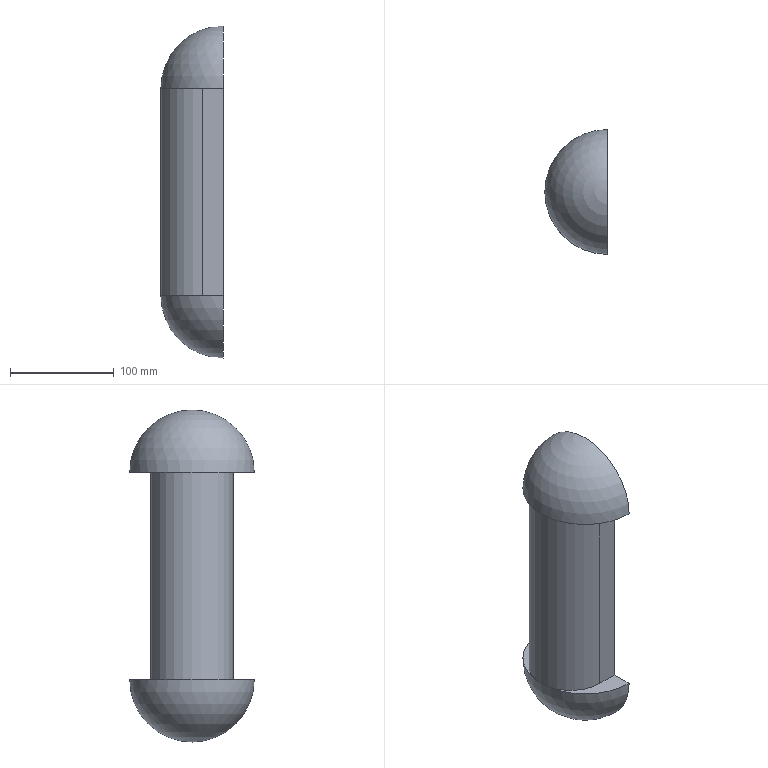Part | SolidWorks | features 3DProfileFeature 1, Extrusion 1, MirrorPattern 1, Revolution 1 | 1 solid | 10 faces | box 60 x 120 x 320 mm | volume 1275044 mm3 | plane 7 | sphere 2 | cylinder 1 | commonest cylinder face diameters 80 x1
STEP:
#1=CARTESIAN_POINT('',(-20.,0.,-100.));
#2=VERTEX_POINT('',#1);
#3=CARTESIAN_POINT('',(-20.,0.,100.));
#4=VERTEX_POINT('',#3);
#5=CARTESIAN_POINT('',(-20.,0.,-100.));
#6=DIRECTION('',(0.,0.,1.));
#7=VECTOR('',#6,1000.);
#8=LINE('',#5,#7);
#9=EDGE_CURVE('',#2,#4,#8,.T.);
#10=ORIENTED_EDGE('',*,*,#9,.T.);
#11=CARTESIAN_POINT('',(0.,0.,100.));
#12=VERTEX_POINT('',#11);
#13=CARTESIAN_POINT('',(0.,0.,100.));
#14=DIRECTION('',(-1.,0.,0.));
#15=VECTOR('',#14,1000.);
#16=LINE('',#13,#15);
#17=EDGE_CURVE('',#12,#4,#16,.T.);
#18=ORIENTED_EDGE('',*,*,#17,.F.);
#19=CARTESIAN_POINT('',(0.,0.,-100.));
#20=VERTEX_POINT('',#19);
#21=CARTESIAN_POINT('',(0.,0.,-100.));
#22=DIRECTION('',(0.,0.,1.));
#23=VECTOR('',#22,1000.);
#24=LINE('',#21,#23);
#25=EDGE_CURVE('',#20,#12,#24,.T.);
#26=ORIENTED_EDGE('',*,*,#25,.F.);
#27=CARTESIAN_POINT('',(0.,0.,-100.));
#28=DIRECTION('',(-1.,0.,0.));
#29=VECTOR('',#28,1000.);
#30=LINE('',#27,#29);
#31=EDGE_CURVE('',#20,#2,#30,.T.);
#32=ORIENTED_EDGE('',*,*,#31,.T.);
#33=EDGE_LOOP('',(#10,#18,#26,#32));
#34=FACE_OUTER_BOUND('',#33,.T.);
#35=CARTESIAN_POINT('',(0.,0.,-100.));
#36=DIRECTION('',(0.,1.,0.));
#37=DIRECTION('',(0.,0.,1.));
#38=AXIS2_PLACEMENT_3D('',#35,#36,#37);
#39=PLANE('',#38);
#40=ADVANCED_FACE('',(#34),#39,.T.);
#41=ORIENTED_EDGE('',*,*,#25,.T.);
#42=CARTESIAN_POINT('',(0.,20.,100.));
#43=VERTEX_POINT('',#42);
#44=CARTESIAN_POINT('',(0.,20.,100.));
#45=DIRECTION('',(0.,-1.,0.));
#46=VECTOR('',#45,1000.);
#47=LINE('',#44,#46);
#48=EDGE_CURVE('',#43,#12,#47,.T.);
#49=ORIENTED_EDGE('',*,*,#48,.F.);
#50=CARTESIAN_POINT('',(0.,-100.,100.));
#51=VERTEX_POINT('',#50);
#52=CARTESIAN_POINT('',(0.,-40.,100.));
#53=DIRECTION('',(-1.,0.,0.));
#54=DIRECTION('',(0.,-1.,0.));
#55=AXIS2_PLACEMENT_3D('',#52,#53,#54);
#56=CIRCLE('',#55,60.);
#57=EDGE_CURVE('',#51,#43,#56,.T.);
#58=ORIENTED_EDGE('',*,*,#57,.F.);
#59=CARTESIAN_POINT('',(0.,-80.,100.));
#60=VERTEX_POINT('',#59);
#61=CARTESIAN_POINT('',(0.,20.,100.));
#62=DIRECTION('',(0.,-1.,0.));
#63=VECTOR('',#62,1000.);
#64=LINE('',#61,#63);
#65=EDGE_CURVE('',#60,#51,#64,.T.);
#66=ORIENTED_EDGE('',*,*,#65,.F.);
#67=CARTESIAN_POINT('',(0.,-80.,-100.));
#68=VERTEX_POINT('',#67);
#69=CARTESIAN_POINT('',(0.,-80.,-100.));
#70=DIRECTION('',(0.,0.,1.));
#71=VECTOR('',#70,1000.);
#72=LINE('',#69,#71);
#73=EDGE_CURVE('',#68,#60,#72,.T.);
#74=ORIENTED_EDGE('',*,*,#73,.F.);
#75=CARTESIAN_POINT('',(0.,-100.,-100.));
#76=VERTEX_POINT('',#75);
#77=CARTESIAN_POINT('',(0.,20.,-100.));
#78=DIRECTION('',(0.,-1.,0.));
#79=VECTOR('',#78,1000.);
#80=LINE('',#77,#79);
#81=EDGE_CURVE('',#68,#76,#80,.T.);
#82=ORIENTED_EDGE('',*,*,#81,.T.);
#83=CARTESIAN_POINT('',(0.,20.,-100.));
#84=VERTEX_POINT('',#83);
#85=CARTESIAN_POINT('',(0.,-40.,-100.));
#86=DIRECTION('',(1.,0.,0.));
#87=DIRECTION('',(0.,-1.,0.));
#88=AXIS2_PLACEMENT_3D('',#85,#86,#87);
#89=CIRCLE('',#88,60.);
#90=EDGE_CURVE('',#76,#84,#89,.T.);
#91=ORIENTED_EDGE('',*,*,#90,.T.);
#92=CARTESIAN_POINT('',(0.,20.,-100.));
#93=DIRECTION('',(0.,-1.,0.));
#94=VECTOR('',#93,1000.);
#95=LINE('',#92,#94);
#96=EDGE_CURVE('',#84,#20,#95,.T.);
#97=ORIENTED_EDGE('',*,*,#96,.T.);
#98=EDGE_LOOP('',(#41,#49,#58,#66,#74,#82,#91,#97));
#99=FACE_OUTER_BOUND('',#98,.T.);
#100=CARTESIAN_POINT('',(0.,0.,-100.));
#101=DIRECTION('',(1.,0.,0.));
#102=DIRECTION('',(0.,1.,0.));
#103=AXIS2_PLACEMENT_3D('',#100,#101,#102);
#104=PLANE('',#103);
#105=ADVANCED_FACE('',(#99),#104,.T.);
#106=ORIENTED_EDGE('',*,*,#73,.T.);
#107=CARTESIAN_POINT('',(-20.,-80.,100.));
#108=VERTEX_POINT('',#107);
#109=CARTESIAN_POINT('',(0.,-80.,100.));
#110=DIRECTION('',(1.,0.,0.));
#111=VECTOR('',#110,1000.);
#112=LINE('',#109,#111);
#113=EDGE_CURVE('',#108,#60,#112,.T.);
#114=ORIENTED_EDGE('',*,*,#113,.F.);
#115=CARTESIAN_POINT('',(-20.,-80.,-100.));
#116=VERTEX_POINT('',#115);
#117=CARTESIAN_POINT('',(-20.,-80.,-100.));
#118=DIRECTION('',(0.,0.,1.));
#119=VECTOR('',#118,1000.);
#120=LINE('',#117,#119);
#121=EDGE_CURVE('',#116,#108,#120,.T.);
#122=ORIENTED_EDGE('',*,*,#121,.F.);
#123=CARTESIAN_POINT('',(0.,-80.,-100.));
#124=DIRECTION('',(1.,0.,0.));
#125=VECTOR('',#124,1000.);
#126=LINE('',#123,#125);
#127=EDGE_CURVE('',#116,#68,#126,.T.);
#128=ORIENTED_EDGE('',*,*,#127,.T.);
#129=EDGE_LOOP('',(#106,#114,#122,#128));
#130=FACE_OUTER_BOUND('',#129,.T.);
#131=CARTESIAN_POINT('',(0.,-80.,-100.));
#132=DIRECTION('',(0.,-1.,0.));
#133=DIRECTION('',(0.,0.,-1.));
#134=AXIS2_PLACEMENT_3D('',#131,#132,#133);
#135=PLANE('',#134);
#136=ADVANCED_FACE('',(#130),#135,.T.);
#137=ORIENTED_EDGE('',*,*,#121,.T.);
#138=CARTESIAN_POINT('',(-60.,-40.,100.));
#139=VERTEX_POINT('',#138);
#140=CARTESIAN_POINT('',(-20.,-40.,100.));
#141=DIRECTION('',(0.,0.,1.));
#142=DIRECTION('',(-1.,0.,0.));
#143=AXIS2_PLACEMENT_3D('',#140,#141,#142);
#144=CIRCLE('',#143,40.);
#145=EDGE_CURVE('',#139,#108,#144,.T.);
#146=ORIENTED_EDGE('',*,*,#145,.F.);
#147=CARTESIAN_POINT('',(-20.,-40.,100.));
#148=DIRECTION('',(0.,0.,1.));
#149=DIRECTION('',(-1.,0.,0.));
#150=AXIS2_PLACEMENT_3D('',#147,#148,#149);
#151=CIRCLE('',#150,40.);
#152=EDGE_CURVE('',#4,#139,#151,.T.);
#153=ORIENTED_EDGE('',*,*,#152,.F.);
#154=ORIENTED_EDGE('',*,*,#9,.F.);
#155=CARTESIAN_POINT('',(-60.,-40.,-100.));
#156=VERTEX_POINT('',#155);
#157=CARTESIAN_POINT('',(-20.,-40.,-100.));
#158=DIRECTION('',(0.,0.,1.));
#159=DIRECTION('',(-1.,0.,0.));
#160=AXIS2_PLACEMENT_3D('',#157,#158,#159);
#161=CIRCLE('',#160,40.);
#162=EDGE_CURVE('',#2,#156,#161,.T.);
#163=ORIENTED_EDGE('',*,*,#162,.T.);
#164=CARTESIAN_POINT('',(-20.,-40.,-100.));
#165=DIRECTION('',(0.,0.,1.));
#166=DIRECTION('',(-1.,0.,0.));
#167=AXIS2_PLACEMENT_3D('',#164,#165,#166);
#168=CIRCLE('',#167,40.);
#169=EDGE_CURVE('',#156,#116,#168,.T.);
#170=ORIENTED_EDGE('',*,*,#169,.T.);
#171=EDGE_LOOP('',(#137,#146,#153,#154,#163,#170));
#172=FACE_OUTER_BOUND('',#171,.T.);
#173=CARTESIAN_POINT('',(-20.,-40.,-100.));
#174=DIRECTION('',(0.,0.,1.));
#175=DIRECTION('',(1.,0.,0.));
#176=AXIS2_PLACEMENT_3D('',#173,#174,#175);
#177=CYLINDRICAL_SURFACE('',#176,40.);
#178=ADVANCED_FACE('',(#172),#177,.T.);
#179=ORIENTED_EDGE('',*,*,#31,.F.);
#180=ORIENTED_EDGE('',*,*,#96,.F.);
#181=CARTESIAN_POINT('',(0.,-40.,-100.));
#182=DIRECTION('',(0.,0.,-1.));
#183=DIRECTION('',(0.,-1.,0.));
#184=AXIS2_PLACEMENT_3D('',#181,#182,#183);
#185=CIRCLE('',#184,60.);
#186=EDGE_CURVE('',#156,#84,#185,.T.);
#187=ORIENTED_EDGE('',*,*,#186,.F.);
#188=ORIENTED_EDGE('',*,*,#162,.F.);
#189=EDGE_LOOP('',(#179,#180,#187,#188));
#190=FACE_OUTER_BOUND('',#189,.T.);
#191=CARTESIAN_POINT('',(0.,-40.,-100.));
#192=DIRECTION('',(0.,0.,1.));
#193=DIRECTION('',(0.,-1.,0.));
#194=AXIS2_PLACEMENT_3D('',#191,#192,#193);
#195=PLANE('',#194);
#196=ADVANCED_FACE('',(#190),#195,.T.);
#197=ORIENTED_EDGE('',*,*,#127,.F.);
#198=ORIENTED_EDGE('',*,*,#169,.F.);
#199=CARTESIAN_POINT('',(0.,-40.,-100.));
#200=DIRECTION('',(0.,0.,-1.));
#201=DIRECTION('',(0.,-1.,0.));
#202=AXIS2_PLACEMENT_3D('',#199,#200,#201);
#203=CIRCLE('',#202,60.);
#204=EDGE_CURVE('',#76,#156,#203,.T.);
#205=ORIENTED_EDGE('',*,*,#204,.F.);
#206=ORIENTED_EDGE('',*,*,#81,.F.);
#207=EDGE_LOOP('',(#197,#198,#205,#206));
#208=FACE_OUTER_BOUND('',#207,.T.);
#209=CARTESIAN_POINT('',(0.,-40.,-100.));
#210=DIRECTION('',(0.,0.,1.));
#211=DIRECTION('',(0.,-1.,0.));
#212=AXIS2_PLACEMENT_3D('',#209,#210,#211);
#213=PLANE('',#212);
#214=ADVANCED_FACE('',(#208),#213,.T.);
#215=ORIENTED_EDGE('',*,*,#90,.F.);
#216=ORIENTED_EDGE('',*,*,#204,.T.);
#217=ORIENTED_EDGE('',*,*,#186,.T.);
#218=EDGE_LOOP('',(#215,#216,#217));
#219=FACE_OUTER_BOUND('',#218,.T.);
#220=CARTESIAN_POINT('',(0.,-40.,-100.));
#221=DIRECTION('',(0.,0.,1.));
#222=DIRECTION('',(1.,0.,0.));
#223=AXIS2_PLACEMENT_3D('',#220,#221,#222);
#224=SPHERICAL_SURFACE('',#223,60.);
#225=ADVANCED_FACE('',(#219),#224,.T.);
#226=ORIENTED_EDGE('',*,*,#48,.T.);
#227=ORIENTED_EDGE('',*,*,#17,.T.);
#228=ORIENTED_EDGE('',*,*,#152,.T.);
#229=CARTESIAN_POINT('',(0.,-40.,100.));
#230=DIRECTION('',(0.,0.,-1.));
#231=DIRECTION('',(0.,-1.,0.));
#232=AXIS2_PLACEMENT_3D('',#229,#230,#231);
#233=CIRCLE('',#232,60.);
#234=EDGE_CURVE('',#139,#43,#233,.T.);
#235=ORIENTED_EDGE('',*,*,#234,.T.);
#236=EDGE_LOOP('',(#226,#227,#228,#235));
#237=FACE_OUTER_BOUND('',#236,.T.);
#238=CARTESIAN_POINT('',(0.,-40.,100.));
#239=DIRECTION('',(0.,0.,-1.));
#240=DIRECTION('',(0.,-1.,0.));
#241=AXIS2_PLACEMENT_3D('',#238,#239,#240);
#242=PLANE('',#241);
#243=ADVANCED_FACE('',(#237),#242,.T.);
#244=CARTESIAN_POINT('',(0.,-40.,100.));
#245=DIRECTION('',(0.,0.,-1.));
#246=DIRECTION('',(0.,-1.,0.));
#247=AXIS2_PLACEMENT_3D('',#244,#245,#246);
#248=CIRCLE('',#247,60.);
#249=EDGE_CURVE('',#51,#139,#248,.T.);
#250=ORIENTED_EDGE('',*,*,#249,.T.);
#251=ORIENTED_EDGE('',*,*,#145,.T.);
#252=ORIENTED_EDGE('',*,*,#113,.T.);
#253=ORIENTED_EDGE('',*,*,#65,.T.);
#254=EDGE_LOOP('',(#250,#251,#252,#253));
#255=FACE_OUTER_BOUND('',#254,.T.);
#256=CARTESIAN_POINT('',(0.,-40.,100.));
#257=DIRECTION('',(0.,0.,-1.));
#258=DIRECTION('',(0.,-1.,0.));
#259=AXIS2_PLACEMENT_3D('',#256,#257,#258);
#260=PLANE('',#259);
#261=ADVANCED_FACE('',(#255),#260,.T.);
#262=ORIENTED_EDGE('',*,*,#57,.T.);
#263=ORIENTED_EDGE('',*,*,#234,.F.);
#264=ORIENTED_EDGE('',*,*,#249,.F.);
#265=EDGE_LOOP('',(#262,#263,#264));
#266=FACE_OUTER_BOUND('',#265,.T.);
#267=CARTESIAN_POINT('',(0.,-40.,100.));
#268=DIRECTION('',(0.,0.,1.));
#269=DIRECTION('',(1.,0.,0.));
#270=AXIS2_PLACEMENT_3D('',#267,#268,#269);
#271=SPHERICAL_SURFACE('',#270,60.);
#272=ADVANCED_FACE('',(#266),#271,.T.);
#273=CLOSED_SHELL('',(#40,#105,#136,#178,#196,#214,#225,#243,#261,#272));
#274=MANIFOLD_SOLID_BREP('',#273);
#275=CARTESIAN_POINT('',(0.,0.,0.));
#276=DIRECTION('',(0.,0.,1.));
#277=DIRECTION('',(1.,0.,0.));
#278=AXIS2_PLACEMENT_3D('',#275,#276,#277);
#279=(LENGTH_UNIT()NAMED_UNIT(*)SI_UNIT(.MILLI.,.METRE.));
#280=UNCERTAINTY_MEASURE_WITH_UNIT(LENGTH_MEASURE(0.00001),#279,'','');
#281=(NAMED_UNIT(*)PLANE_ANGLE_UNIT()SI_UNIT($,.RADIAN.));
#282=(NAMED_UNIT(*)SI_UNIT($,.STERADIAN.)SOLID_ANGLE_UNIT());
#283=(GEOMETRIC_REPRESENTATION_CONTEXT(3)GLOBAL_UNCERTAINTY_ASSIGNED_CONTEXT((#280))GLOBAL_UNIT_ASSIGNED_CONTEXT((#279,#281,#282))REPRESENTATION_CONTEXT('',''));
#284=ADVANCED_BREP_SHAPE_REPRESENTATION('',(#274,#278),#283);